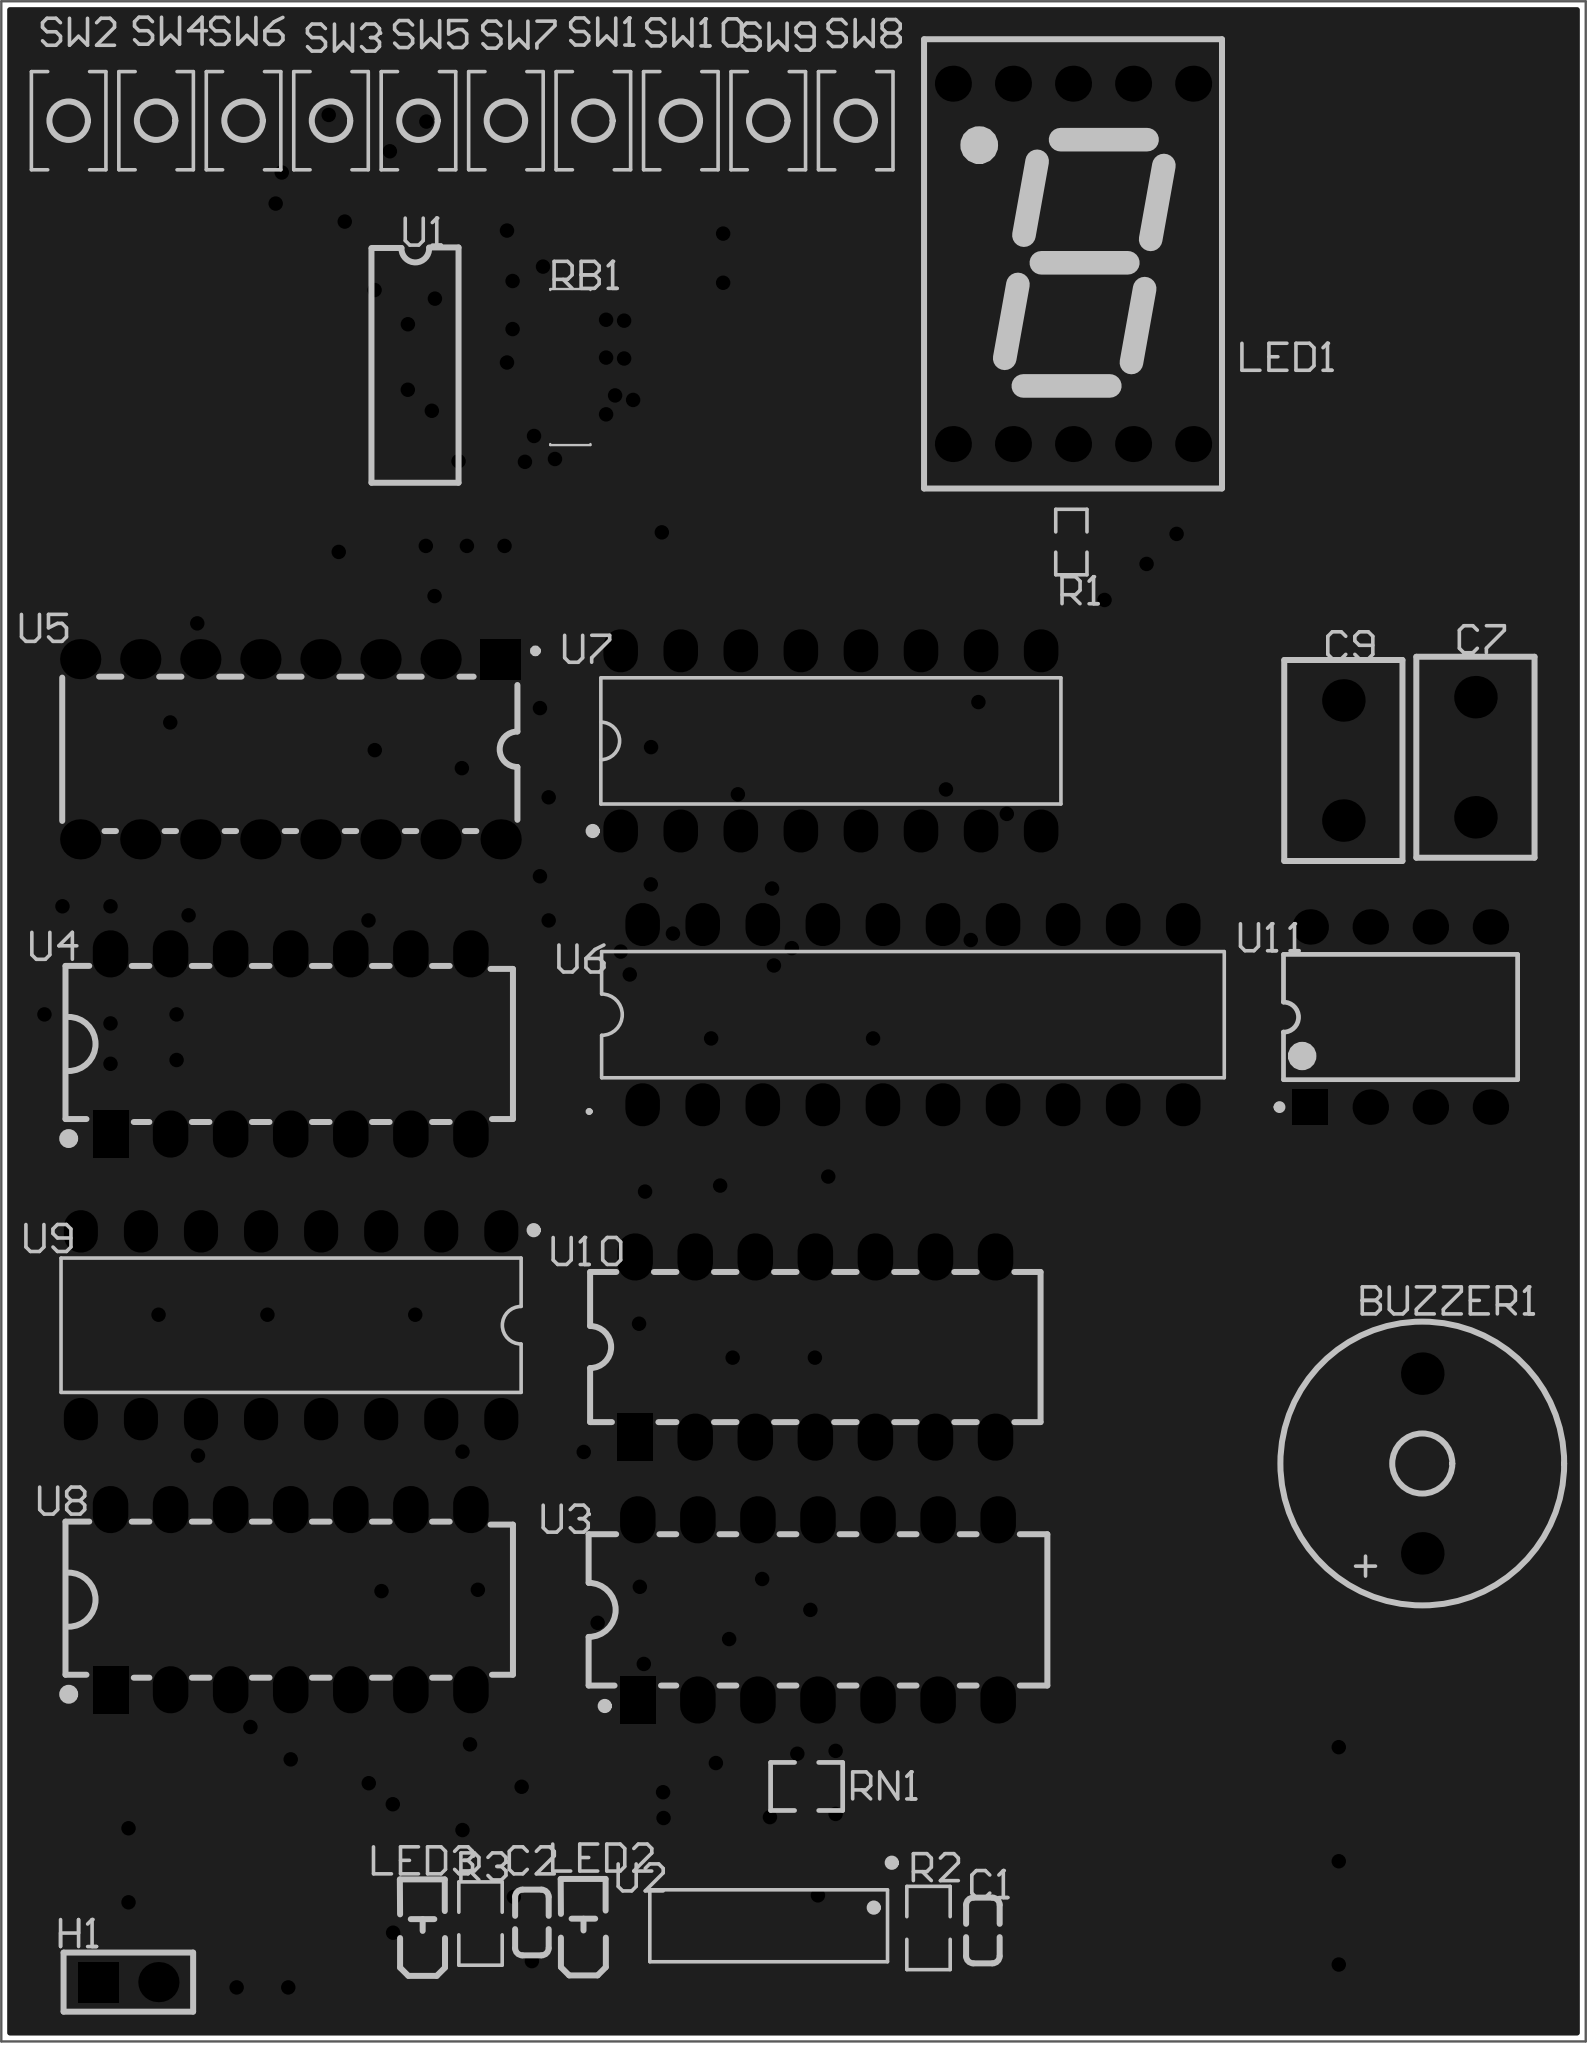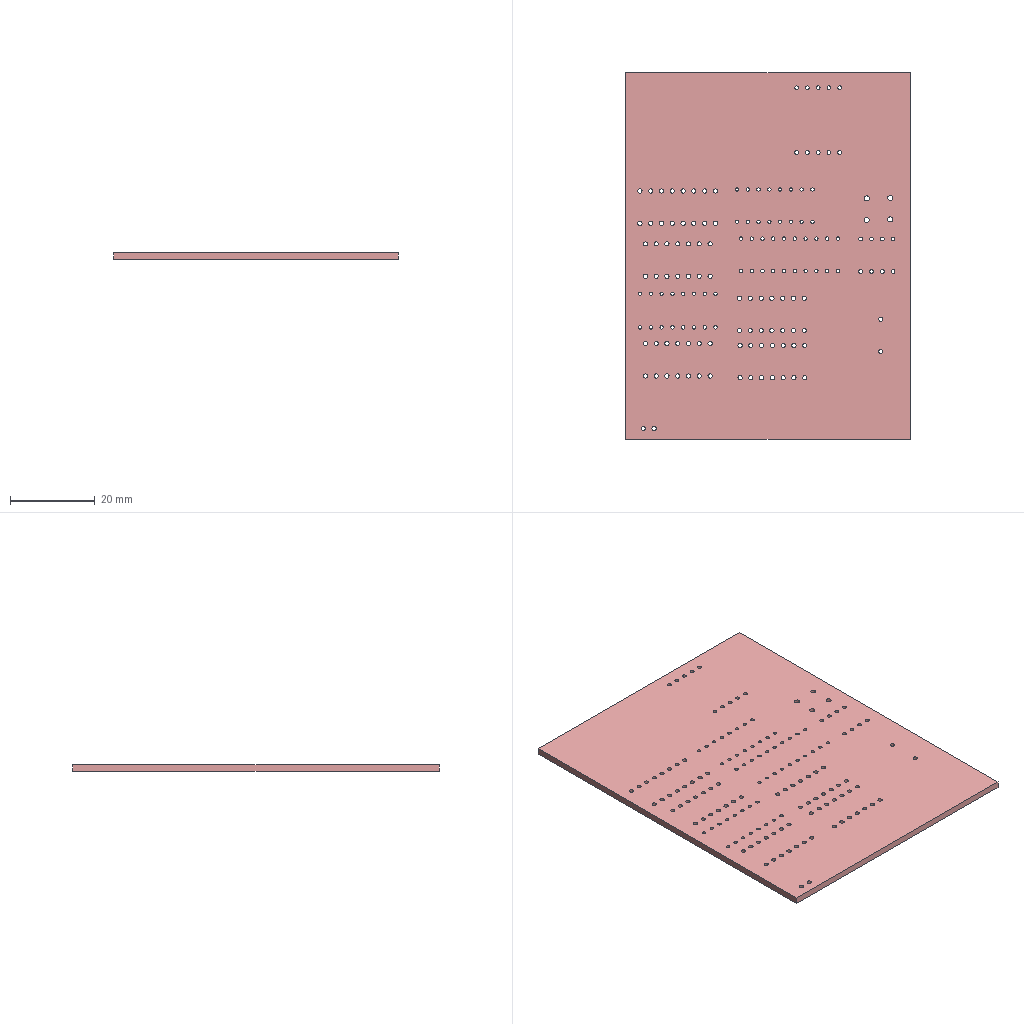Circuit board layout | Altium Designer | box 67 x 86.3 x 1.6 mm
Layer stack:
# Altium Designer layer stack of  (unit mm; dielectric type: 0 none, 1 core, 2 prepreg, 3 surface material)
index,name,kind,layer,copper_thickness_mm,dielectric_type,dielectric_thickness_mm,dielectric_material,dielectric_constant
0,Top Paste Mask Layer,other,,,,,,
1,Top Silkscreen Layer,other,,,,,,
2,Top Solder Mask Layer,dielectric,,,3,0.01,,3.3
3,Top Layer,copper,Top Layer,0.035,,,,
4,Dielectric1,dielectric,,,3,1.51,FR4,4.5
5,Bottom Layer,copper,Bottom Layer,0.035,,,,
6,Bottom Solder Mask Layer,dielectric,,,3,0.01,,3.3
7,Bottom Silkscreen Layer,other,,,,,,
8,Bottom Paste Mask Layer,other,,,,,,
# drill layer pairs: low layer,high layer
drill_pair,Top Layer,Bottom Layer
Part placement:
Designator,Comment,Layer,Footprint,Center-X(mm),Center-Y(mm),Rotation
H1,,TopLayer,HDR-TH_2P-P2.54-V-F,86.988,81.377,0
C7,C104,TopLayer,CAP-TH_L8.5-W5.0-P5.00-D1.2,143.956,133.177,270
C9,C103,TopLayer,CAP-TH_L8.5-W5.0-P5.00-D1.2,138.37,133.038,270
U11,100kHz,TopLayer,DIP-8_L9.8-W6.6-P2.54-LS7.6-BL,140.779,122.19,0
BUZZER1,2.4kHz,TopLayer,BUZ-TH_BD12.0-P7.60-D0.6-FD,141.707,103.308,90
C1,1uF,TopLayer,C0603,123.125,83.56,90
C2,10uF,TopLayer,C0603,104.054,83.898,90
LED1,,TopLayer,LED-SEG-TH_10P-L12.6-W19.0-P2.54-S15.24-BL,126.937,154.04,180
LED2,,TopLayer,LED_0805,106.231,83.76,90
LED3,,TopLayer,LED_0805,99.429,83.741,90
R1,50Ω,TopLayer,R0603,126.867,142.277,90
R2,100K,TopLayer,R0805,120.826,83.666,90
R3,72K,TopLayer,R0805,101.88,83.854,90
RB1,10kΩ,TopLayer,RES-ARRAY-SMD_0603-16P-L6.4-W1.6-TL,105.729,149.677,270
RN1,10kΩ,TopLayer,RES-ARRAY-SMD_0603-4P-L1.6-W1.6-BL,115.672,89.651,90
SW1,,TopLayer,Key_SMD_3x4x2,106.653,160.096,270
SW2,,TopLayer,Key_SMD_3x4x2,84.463,160.096,270
SW3,,TopLayer,Key_SMD_3x4x2,102.954,160.096,270
SW4,,TopLayer,Key_SMD_3x4x2,88.161,160.096,90
SW5,,TopLayer,Key_SMD_3x4x2,99.256,160.096,90
SW6,,TopLayer,Key_SMD_3x4x2,91.859,160.096,270
SW7,,TopLayer,Key_SMD_3x4x2,95.558,160.096,270
SW8,,TopLayer,Key_SMD_3x4x2,117.748,160.096,270
SW9,,TopLayer,Key_SMD_3x4x2,114.049,160.096,270
SW10,,TopLayer,Key_SMD_3x4x2,110.351,160.096,270
U1,SN74LS148DR(LX),TopLayer,SOIC-16_L9.9-W3.9-P1.27-LS6.0-BL-1,99.123,149.76,270
U2,SN74LS279D,TopLayer,SOIC-16_L9.9-W3.9-P1.27-LS6.0-BL,114.066,83.759,180
U3,SN74LS08N,TopLayer,PDIP-14_L19.3-W6.4-P2.54-LS7.9-BL-1,116.152,97.119,0
U4,SN74LS04N(LX),TopLayer,DIP-14_L19.1-W6.4-P2.54-LS7.6-BL,93.854,121.051,0
U5,XD74LS83,TopLayer,PDIP-16_L19.1-W6.4-P2.54-LS7.62-BL,93.841,133.514,180
U6,SN74LS373N(LX),TopLayer,PDIP-20_L26.2-W7.6-P2.54-LS7.9-BL,120.167,122.29,0
U7,XD74LS48,TopLayer,DIP-16_L19.3-W6.4-P2.54-LS7.6-BL,116.698,133.867,0
U8,SN74LS04N(LX),TopLayer,DIP-14_L19.1-W6.4-P2.54-LS7.6-BL,93.854,97.55,0
U9,SN74LS279AN(LX),TopLayer,PDIP-16_L19.3-W6.4-P2.54-LS7.94-BL,93.869,109.156,180
U10,SN74LS00N(XBLW),TopLayer,PDIP-14_L19.3-W6.4-P2.54-LS7.6-BL,116.04,108.234,0
Pad and via stacks:
# Altium Designer via and pad stacks of  (unit mm). Each distinct definition once, with the count of objects using it.
# via: kind,start_layer,end_layer,hole_mm,diameter_mm,mode(0 simple;1 top-mid-bottom;2 full stack),diameter_per_layer,count,example_net
# pad: kind,layer,hole_mm,hole_type(0 round;1 square;2 slot),plating,top_size,top_shape(1 round;2 rect;3 octagon;9 rounded rect),mid_size,bottom_size,mode,footprint,size_per_layer,count,example
pad,Multi-Layer,1,0,plated,1.7x1.7,2,1.7x1.7,1.7x1.7,0,HDR-TH_2P-P2.54-V-F,,1,H1.1
pad,Multi-Layer,1,0,plated,1.7x1.7,1,1.7x1.7,1.7x1.7,0,HDR-TH_2P-P2.54-V-F,,1,H1.2
pad,Multi-Layer,1.2,0,plated,1.8x1.8,1,1.8x1.8,1.8x1.8,0,CAP-TH_L8.5-W5.0-P5.00-D1.2,,4,C7.1
pad,Multi-Layer,0.9,0,plated,1.5x1.5,2,1.5x1.5,1.5x1.5,0,DIP-8_L9.8-W6.6-P2.54-LS7.6-BL,,1,U11.1
pad,Multi-Layer,0.9,0,plated,1.5x1.5,1,1.5x1.5,1.5x1.5,0,DIP-8_L9.8-W6.6-P2.54-LS7.6-BL,,7,U11.2
pad,Multi-Layer,1,0,plated,1.8x1.8,1,1.8x1.8,1.8x1.8,0,BUZ-TH_BD12.0-P7.60-D0.6-FD,,2,BUZZER1.2
pad,Multi-Layer,0.9144,0,plated,1.524x1.524,1,1.524x1.524,1.524x1.524,0,LED-SEG-TH_10P-L12.6-W19.0-P2.54-S15.24-BL,,10,LED1.1
pad,Multi-Layer,1,0,plated,2x1.5,2,2x1.5,2x1.5,0,PDIP-14_L19.3-W6.4-P2.54-LS7.9-BL-1,,1,U3.1
pad,Multi-Layer,1,0,plated,2x1.5,1,2x1.5,2x1.5,0,PDIP-14_L19.3-W6.4-P2.54-LS7.9-BL-1,,13,U3.2
pad,Multi-Layer,1,0,plated,2x1.5,1,2x1.5,2x1.5,0,DIP-14_L19.1-W6.4-P2.54-LS7.6-BL,,26,U4.8
pad,Multi-Layer,1,0,plated,2x1.5,2,2x1.5,2x1.5,0,DIP-14_L19.1-W6.4-P2.54-LS7.6-BL,,2,U4.1
pad,Multi-Layer,1,0,plated,1.7x1.7,2,1.7x1.7,1.7x1.7,0,PDIP-16_L19.1-W6.4-P2.54-LS7.62-BL,,1,U5.1
pad,Multi-Layer,1,0,plated,1.7x1.7,1,1.7x1.7,1.7x1.7,0,PDIP-16_L19.1-W6.4-P2.54-LS7.62-BL,,15,U5.2
pad,Multi-Layer,0.8,0,plated,1.46x1.825,1,1.46x1.825,1.46x1.825,0,PDIP-20_L26.2-W7.6-P2.54-LS7.9-BL,,20,U6.1
pad,Multi-Layer,0.8,0,plated,1.46x1.825,1,1.46x1.825,1.46x1.825,0,DIP-16_L19.3-W6.4-P2.54-LS7.6-BL,,16,U7.9
pad,Multi-Layer,0.8,0,plated,1.44x1.8,1,1.44x1.8,1.44x1.8,0,PDIP-16_L19.3-W6.4-P2.54-LS7.94-BL,,16,U9.1
pad,Multi-Layer,1,0,plated,1.5x2,2,1.5x2,1.5x2,0,PDIP-14_L19.3-W6.4-P2.54-LS7.6-BL,,1,U10.1
pad,Multi-Layer,1,0,plated,1.5x2,1,1.5x2,1.5x2,0,PDIP-14_L19.3-W6.4-P2.54-LS7.6-BL,,13,U10.2
pad,Top Layer,0,0,plated,0.8x0.9,2,0.8x0.9,0.8x0.9,0,C0603,,4,C1.2
pad,Top Layer,0,0,plated,1x1.25,2,1x1.25,1x1.25,0,LED_0805,,4,LED2.2
pad,Top Layer,0,0,plated,0.8065x0.864,2,0.8065x0.864,0.8065x0.864,0,R0603,,2,R1.2
pad,Top Layer,0,0,plated,1.133x1.377,2,1.133x1.377,1.133x1.377,0,R0805,,4,R2.2
pad,Top Layer,0,0,plated,0.6x0.8,2,0.6x0.8,0.6x0.8,0,RES-ARRAY-SMD_0603-16P-L6.4-W1.6-TL,,16,RB1.1
pad,Top Layer,0,0,plated,0.8x0.6,2,0.8x0.6,0.8x0.6,0,RES-ARRAY-SMD_0603-4P-L1.6-W1.6-BL,,4,RN1.1
pad,Top Layer,0,0,plated,1.53x1.36,2,1.53x1.36,1.53x1.36,0,Key_SMD_3x4x2,,20,SW1.1
pad,Top Layer,0,0,plated,0.6x1.8,1,0.6x1.8,0.6x1.8,0,SOIC-16_L9.9-W3.9-P1.27-LS6.0-BL-1,,16,U1.9
pad,Top Layer,0,0,plated,0.602x1.971,1,0.602x1.971,0.602x1.971,0,SOIC-16_L9.9-W3.9-P1.27-LS6.0-BL,,16,U2.1
via,Top Layer,Bottom Layer,0.3048,0.6096,0,,115,
Copper pours:
name,layer,net,type(0 solid;1 hatched;2 none)
Top Layer-GND,Top Layer,GND,0
Bottom Layer-GND,Bottom Layer,GND,0
Design rules, without the lines most boards share:
# Altium Designer design rules of  (exported by Altium Designer, unit mm)
# columns: name | kind | enabled | priority | scope1 | scope2 | descriptor | typed fields (field=value)
copperThickness2oz | 0 | disabled | 1 | All | All | Clearance Constraint (Gap=6mil) (Disabled)(All),(All) | gap=0.1524
Plane_innerPlane | 0 | disabled | 2 | All | All | Clearance Constraint (Gap=6mil) (Disabled)(All),(All) | gap=0.1524
Copper_copperRegion | 0 | disabled | 3 | All | All | Clearance Constraint (Gap=6mil) (Disabled)(All),(All) | gap=0.1524
copperThickness1oz | 0 | enabled | 4 | All | All | Clearance Constraint (Gap=6mil) (All),(All) | gap=0.1524
otherClearance | 52 | enabled | 1 | All | All | Hole To Hole Clearance (Gap=11.8mil) (All),(All) | gap=0.2997
POWER | 2 | enabled | 2 | (InNet('GND') OR InNet('+5V')) | All | Width Constraint (Min=5mil) (Max=100mil) (Preferred=30mil) ((InNet('GND') OR InNet('+5V'))) |
copperThickness1oz_2 | 2 | enabled | 3 | All | All | Width Constraint (Min=5mil) (Max=100mil) (Preferred=10mil) (All) |
viaSize | 11 | enabled | 1 | All | All | Routing Via (MinHoleWidth=11.8mil) (MaxHoleWidth=248mil) (PreferredHoleWidth=12mil) (MinWidth=19.7mil) (MaxWidth=393.7mil) (PreferedWidth=24mil) (All) | via_min_hole=0.2997 via_max_hole=6.299 via_preferred_diameter=0.6096 via_preferred_hole=0.3048
copperRegion | 20 | enabled | 1 | All | All | Polygon Connect Rule(Direct Connect )(Conductor Width=10mil) (Relief Angle=90 Angle) (Entries=4) (Air Gap Width=10mil) (All),(All) | connect_style(0=relief,1=direct,2=none)=1 relief_conductor_width=0.254 relief_entries=4